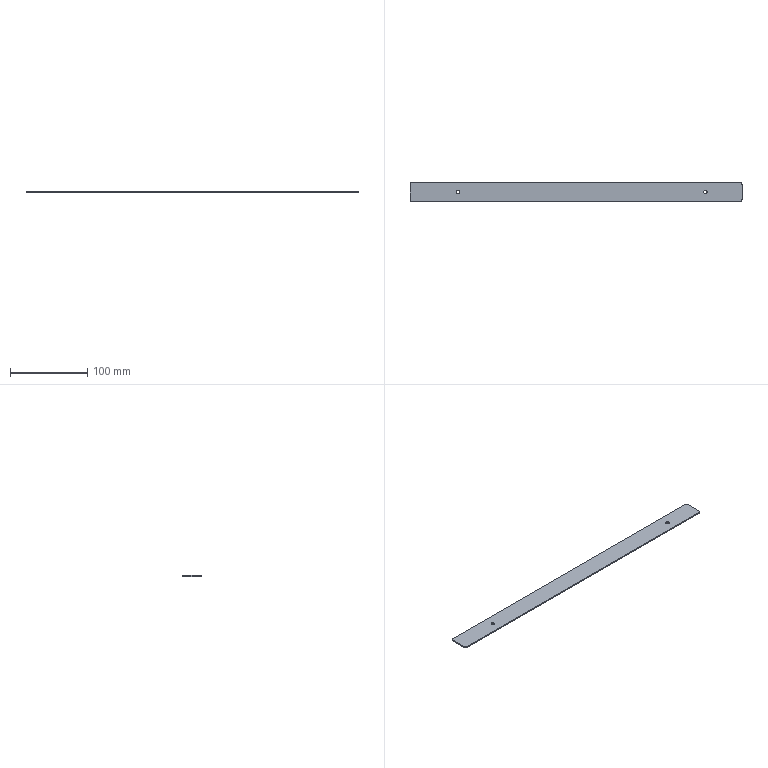Part | STEP file | 1 solid | 14 faces | box 430 x 25 x 1.5 mm | volume 16066 mm3 | cylinder 8 | plane 6 | commonest cylinder face diameters 4.5 x4 6 x4
STEP:
#1=CARTESIAN_POINT('',(0.,0.,0.));
#2=DIRECTION('',(0.,0.,1.));
#3=DIRECTION('',(1.,0.,0.));
#4=AXIS2_PLACEMENT_3D('',#1,#2,#3);
#5=CARTESIAN_POINT('',(-108.085,-48.,1.5));
#6=VERTEX_POINT('',#5);
#7=CARTESIAN_POINT('',(-111.085,-45.,1.5));
#8=VERTEX_POINT('',#7);
#9=CARTESIAN_POINT('',(-111.085,-48.,1.5));
#10=DIRECTION('',(0.,0.,1.));
#11=DIRECTION('',(1.,0.,0.));
#12=AXIS2_PLACEMENT_3D('',#9,#10,#11);
#13=CIRCLE('',#12,3.);
#14=CARTESIAN_POINT('',(-111.085,-48.,1.5));
#15=DIRECTION('',(0.,0.,-1.));
#16=DIRECTION('',(-1.,0.,0.));
#17=AXIS2_PLACEMENT_3D('',#14,#15,#16);
#18=CYLINDRICAL_SURFACE('',#17,3.);
#19=CARTESIAN_POINT('',(3.142,0.));
#20=DIRECTION('',(-1.,0.));
#21=VECTOR('',#20,1.);
#22=LINE('',#19,#21);
#23=(GEOMETRIC_REPRESENTATION_CONTEXT(2)PARAMETRIC_REPRESENTATION_CONTEXT()REPRESENTATION_CONTEXT('',''));
#24=DEFINITIONAL_REPRESENTATION('',(#22),#23);
#25=PCURVE('',#18,#24);
#26=CARTESIAN_POINT('',(0.,0.,1.5));
#27=DIRECTION('',(0.,0.,1.));
#28=DIRECTION('',(1.,0.,0.));
#29=AXIS2_PLACEMENT_3D('',#26,#27,#28);
#30=PLANE('',#29);
#31=CARTESIAN_POINT('',(-111.085,-48.));
#32=DIRECTION('',(1.,0.));
#33=AXIS2_PLACEMENT_2D('',#31,#32);
#34=CIRCLE('',#33,3.);
#35=(GEOMETRIC_REPRESENTATION_CONTEXT(2)PARAMETRIC_REPRESENTATION_CONTEXT()REPRESENTATION_CONTEXT('',''));
#36=DEFINITIONAL_REPRESENTATION('',(#34),#35);
#37=PCURVE('',#30,#36);
#38=SURFACE_CURVE('',#13,(#25,#37),.PCURVE_S1.);
#39=EDGE_CURVE('',#6,#8,#38,.T.);
#40=ORIENTED_EDGE('',*,*,#39,.F.);
#41=CARTESIAN_POINT('',(-108.085,-48.,0.));
#42=VERTEX_POINT('',#41);
#43=CARTESIAN_POINT('',(-108.085,-48.,1.5));
#44=DIRECTION('',(0.,0.,1.));
#45=VECTOR('',#44,1.);
#46=LINE('',#43,#45);
#47=CARTESIAN_POINT('',(3.142,0.));
#48=DIRECTION('',(0.,-1.));
#49=VECTOR('',#48,1.);
#50=LINE('',#47,#49);
#51=(GEOMETRIC_REPRESENTATION_CONTEXT(2)PARAMETRIC_REPRESENTATION_CONTEXT()REPRESENTATION_CONTEXT('',''));
#52=DEFINITIONAL_REPRESENTATION('',(#50),#51);
#53=PCURVE('',#18,#52);
#54=CARTESIAN_POINT('',(-108.085,-70.,1.5));
#55=DIRECTION('',(-1.,0.,0.));
#56=DIRECTION('',(0.,0.,1.));
#57=AXIS2_PLACEMENT_3D('',#54,#55,#56);
#58=PLANE('',#57);
#59=CARTESIAN_POINT('',(0.,22.));
#60=DIRECTION('',(1.,0.));
#61=VECTOR('',#60,1.);
#62=LINE('',#59,#61);
#63=(GEOMETRIC_REPRESENTATION_CONTEXT(2)PARAMETRIC_REPRESENTATION_CONTEXT()REPRESENTATION_CONTEXT('',''));
#64=DEFINITIONAL_REPRESENTATION('',(#62),#63);
#65=PCURVE('',#58,#64);
#66=SURFACE_CURVE('',#46,(#53,#65),.PCURVE_S1.);
#67=EDGE_CURVE('',#42,#6,#66,.T.);
#68=ORIENTED_EDGE('',*,*,#67,.F.);
#69=CARTESIAN_POINT('',(-111.085,-45.,0.));
#70=VERTEX_POINT('',#69);
#71=CARTESIAN_POINT('',(-111.085,-48.,0.));
#72=DIRECTION('',(0.,0.,-1.));
#73=DIRECTION('',(1.,0.,0.));
#74=AXIS2_PLACEMENT_3D('',#71,#72,#73);
#75=CIRCLE('',#74,3.);
#76=CARTESIAN_POINT('',(-3.142,1.5));
#77=DIRECTION('',(1.,0.));
#78=VECTOR('',#77,1.);
#79=LINE('',#76,#78);
#80=(GEOMETRIC_REPRESENTATION_CONTEXT(2)PARAMETRIC_REPRESENTATION_CONTEXT()REPRESENTATION_CONTEXT('',''));
#81=DEFINITIONAL_REPRESENTATION('',(#79),#80);
#82=PCURVE('',#18,#81);
#83=CARTESIAN_POINT('',(0.,0.,0.));
#84=DIRECTION('',(0.,0.,1.));
#85=DIRECTION('',(1.,0.,0.));
#86=AXIS2_PLACEMENT_3D('',#83,#84,#85);
#87=PLANE('',#86);
#88=CARTESIAN_POINT('',(-108.085,-48.));
#89=CARTESIAN_POINT('',(-108.085,-53.196));
#90=CARTESIAN_POINT('',(-112.585,-50.598));
#91=CARTESIAN_POINT('',(-117.085,-48.));
#92=CARTESIAN_POINT('',(-112.585,-45.402));
#93=CARTESIAN_POINT('',(-108.085,-42.804));
#94=CARTESIAN_POINT('',(-108.085,-48.));
#95=(BOUNDED_CURVE()B_SPLINE_CURVE(2,(#88,#89,#90,#91,#92,#93,#94),.UNSPECIFIED.,.T.,.F.)B_SPLINE_CURVE_WITH_KNOTS((1,2,2,2,2,1),(-2.094,0.,2.094,4.189,6.283,8.378),.UNSPECIFIED.)CURVE()GEOMETRIC_REPRESENTATION_ITEM()RATIONAL_B_SPLINE_CURVE((1.,0.5,1.,0.5,1.,0.5,1.))REPRESENTATION_ITEM(''));
#96=(GEOMETRIC_REPRESENTATION_CONTEXT(2)PARAMETRIC_REPRESENTATION_CONTEXT()REPRESENTATION_CONTEXT('',''));
#97=DEFINITIONAL_REPRESENTATION('',(#95),#96);
#98=PCURVE('',#87,#97);
#99=SURFACE_CURVE('',#75,(#82,#98),.PCURVE_S1.);
#100=EDGE_CURVE('',#70,#42,#99,.T.);
#101=ORIENTED_EDGE('',*,*,#100,.F.);
#102=CARTESIAN_POINT('',(-111.085,-45.,1.5));
#103=DIRECTION('',(0.,0.,-1.));
#104=VECTOR('',#103,1.);
#105=LINE('',#102,#104);
#106=CARTESIAN_POINT('',(1.571,0.));
#107=DIRECTION('',(0.,1.));
#108=VECTOR('',#107,1.);
#109=LINE('',#106,#108);
#110=(GEOMETRIC_REPRESENTATION_CONTEXT(2)PARAMETRIC_REPRESENTATION_CONTEXT()REPRESENTATION_CONTEXT('',''));
#111=DEFINITIONAL_REPRESENTATION('',(#109),#110);
#112=PCURVE('',#18,#111);
#113=CARTESIAN_POINT('',(-108.085,-45.,1.5));
#114=DIRECTION('',(0.,-1.,0.));
#115=DIRECTION('',(-1.,0.,0.));
#116=AXIS2_PLACEMENT_3D('',#113,#114,#115);
#117=PLANE('',#116);
#118=CARTESIAN_POINT('',(3.,0.));
#119=DIRECTION('',(0.,1.));
#120=VECTOR('',#119,1.);
#121=LINE('',#118,#120);
#122=(GEOMETRIC_REPRESENTATION_CONTEXT(2)PARAMETRIC_REPRESENTATION_CONTEXT()REPRESENTATION_CONTEXT('',''));
#123=DEFINITIONAL_REPRESENTATION('',(#121),#122);
#124=PCURVE('',#117,#123);
#125=SURFACE_CURVE('',#105,(#112,#124),.PCURVE_S1.);
#126=EDGE_CURVE('',#8,#70,#125,.T.);
#127=ORIENTED_EDGE('',*,*,#126,.F.);
#128=EDGE_LOOP('',(#40,#68,#101,#127));
#129=FACE_BOUND('',#128,.T.);
#130=ADVANCED_FACE('',(#129),#18,.T.);
#131=CARTESIAN_POINT('',(-111.085,-70.,1.5));
#132=VERTEX_POINT('',#131);
#133=CARTESIAN_POINT('',(-108.085,-67.,1.5));
#134=VERTEX_POINT('',#133);
#135=CARTESIAN_POINT('',(-111.085,-67.,1.5));
#136=DIRECTION('',(0.,0.,1.));
#137=DIRECTION('',(1.,0.,0.));
#138=AXIS2_PLACEMENT_3D('',#135,#136,#137);
#139=CIRCLE('',#138,3.);
#140=CARTESIAN_POINT('',(-111.085,-67.,1.5));
#141=DIRECTION('',(0.,0.,-1.));
#142=DIRECTION('',(-1.,0.,0.));
#143=AXIS2_PLACEMENT_3D('',#140,#141,#142);
#144=CYLINDRICAL_SURFACE('',#143,3.);
#145=CARTESIAN_POINT('',(9.425,0.));
#146=DIRECTION('',(-1.,0.));
#147=VECTOR('',#146,1.);
#148=LINE('',#145,#147);
#149=(GEOMETRIC_REPRESENTATION_CONTEXT(2)PARAMETRIC_REPRESENTATION_CONTEXT()REPRESENTATION_CONTEXT('',''));
#150=DEFINITIONAL_REPRESENTATION('',(#148),#149);
#151=PCURVE('',#144,#150);
#152=CARTESIAN_POINT('',(-111.085,-67.));
#153=DIRECTION('',(1.,0.));
#154=AXIS2_PLACEMENT_2D('',#152,#153);
#155=CIRCLE('',#154,3.);
#156=(GEOMETRIC_REPRESENTATION_CONTEXT(2)PARAMETRIC_REPRESENTATION_CONTEXT()REPRESENTATION_CONTEXT('',''));
#157=DEFINITIONAL_REPRESENTATION('',(#155),#156);
#158=PCURVE('',#30,#157);
#159=SURFACE_CURVE('',#139,(#151,#158),.PCURVE_S1.);
#160=EDGE_CURVE('',#132,#134,#159,.T.);
#161=ORIENTED_EDGE('',*,*,#160,.F.);
#162=CARTESIAN_POINT('',(-111.085,-70.,0.));
#163=VERTEX_POINT('',#162);
#164=CARTESIAN_POINT('',(-111.085,-70.,1.5));
#165=DIRECTION('',(0.,0.,1.));
#166=VECTOR('',#165,1.);
#167=LINE('',#164,#166);
#168=CARTESIAN_POINT('',(4.712,0.));
#169=DIRECTION('',(0.,-1.));
#170=VECTOR('',#169,1.);
#171=LINE('',#168,#170);
#172=(GEOMETRIC_REPRESENTATION_CONTEXT(2)PARAMETRIC_REPRESENTATION_CONTEXT()REPRESENTATION_CONTEXT('',''));
#173=DEFINITIONAL_REPRESENTATION('',(#171),#172);
#174=PCURVE('',#144,#173);
#175=CARTESIAN_POINT('',(-558.085,-70.,1.5));
#176=DIRECTION('',(0.,1.,0.));
#177=DIRECTION('',(1.,0.,0.));
#178=AXIS2_PLACEMENT_3D('',#175,#176,#177);
#179=PLANE('',#178);
#180=CARTESIAN_POINT('',(447.,0.));
#181=DIRECTION('',(0.,-1.));
#182=VECTOR('',#181,1.);
#183=LINE('',#180,#182);
#184=(GEOMETRIC_REPRESENTATION_CONTEXT(2)PARAMETRIC_REPRESENTATION_CONTEXT()REPRESENTATION_CONTEXT('',''));
#185=DEFINITIONAL_REPRESENTATION('',(#183),#184);
#186=PCURVE('',#179,#185);
#187=SURFACE_CURVE('',#167,(#174,#186),.PCURVE_S1.);
#188=EDGE_CURVE('',#163,#132,#187,.T.);
#189=ORIENTED_EDGE('',*,*,#188,.F.);
#190=CARTESIAN_POINT('',(-108.085,-67.,0.));
#191=VERTEX_POINT('',#190);
#192=CARTESIAN_POINT('',(-111.085,-67.,0.));
#193=DIRECTION('',(0.,0.,-1.));
#194=DIRECTION('',(1.,0.,0.));
#195=AXIS2_PLACEMENT_3D('',#192,#193,#194);
#196=CIRCLE('',#195,3.);
#197=CARTESIAN_POINT('',(3.142,1.5));
#198=DIRECTION('',(1.,0.));
#199=VECTOR('',#198,1.);
#200=LINE('',#197,#199);
#201=(GEOMETRIC_REPRESENTATION_CONTEXT(2)PARAMETRIC_REPRESENTATION_CONTEXT()REPRESENTATION_CONTEXT('',''));
#202=DEFINITIONAL_REPRESENTATION('',(#200),#201);
#203=PCURVE('',#144,#202);
#204=CARTESIAN_POINT('',(-108.085,-67.));
#205=CARTESIAN_POINT('',(-108.085,-72.196));
#206=CARTESIAN_POINT('',(-112.585,-69.598));
#207=CARTESIAN_POINT('',(-117.085,-67.));
#208=CARTESIAN_POINT('',(-112.585,-64.402));
#209=CARTESIAN_POINT('',(-108.085,-61.804));
#210=CARTESIAN_POINT('',(-108.085,-67.));
#211=(BOUNDED_CURVE()B_SPLINE_CURVE(2,(#204,#205,#206,#207,#208,#209,#210),.UNSPECIFIED.,.T.,.F.)B_SPLINE_CURVE_WITH_KNOTS((1,2,2,2,2,1),(-2.094,0.,2.094,4.189,6.283,8.378),.UNSPECIFIED.)CURVE()GEOMETRIC_REPRESENTATION_ITEM()RATIONAL_B_SPLINE_CURVE((1.,0.5,1.,0.5,1.,0.5,1.))REPRESENTATION_ITEM(''));
#212=(GEOMETRIC_REPRESENTATION_CONTEXT(2)PARAMETRIC_REPRESENTATION_CONTEXT()REPRESENTATION_CONTEXT('',''));
#213=DEFINITIONAL_REPRESENTATION('',(#211),#212);
#214=PCURVE('',#87,#213);
#215=SURFACE_CURVE('',#196,(#203,#214),.PCURVE_S1.);
#216=EDGE_CURVE('',#191,#163,#215,.T.);
#217=ORIENTED_EDGE('',*,*,#216,.F.);
#218=CARTESIAN_POINT('',(-108.085,-67.,1.5));
#219=DIRECTION('',(0.,0.,-1.));
#220=VECTOR('',#219,1.);
#221=LINE('',#218,#220);
#222=CARTESIAN_POINT('',(3.142,0.));
#223=DIRECTION('',(0.,1.));
#224=VECTOR('',#223,1.);
#225=LINE('',#222,#224);
#226=(GEOMETRIC_REPRESENTATION_CONTEXT(2)PARAMETRIC_REPRESENTATION_CONTEXT()REPRESENTATION_CONTEXT('',''));
#227=DEFINITIONAL_REPRESENTATION('',(#225),#226);
#228=PCURVE('',#144,#227);
#229=CARTESIAN_POINT('',(0.,3.));
#230=DIRECTION('',(-1.,0.));
#231=VECTOR('',#230,1.);
#232=LINE('',#229,#231);
#233=(GEOMETRIC_REPRESENTATION_CONTEXT(2)PARAMETRIC_REPRESENTATION_CONTEXT()REPRESENTATION_CONTEXT('',''));
#234=DEFINITIONAL_REPRESENTATION('',(#232),#233);
#235=PCURVE('',#58,#234);
#236=SURFACE_CURVE('',#221,(#228,#235),.PCURVE_S1.);
#237=EDGE_CURVE('',#134,#191,#236,.T.);
#238=ORIENTED_EDGE('',*,*,#237,.F.);
#239=EDGE_LOOP('',(#161,#189,#217,#238));
#240=FACE_BOUND('',#239,.T.);
#241=ADVANCED_FACE('',(#240),#144,.T.);
#242=CARTESIAN_POINT('',(-535.085,-45.,1.5));
#243=VERTEX_POINT('',#242);
#244=CARTESIAN_POINT('',(-538.085,-48.,1.5));
#245=VERTEX_POINT('',#244);
#246=CARTESIAN_POINT('',(-535.085,-48.,1.5));
#247=DIRECTION('',(0.,0.,1.));
#248=DIRECTION('',(1.,0.,0.));
#249=AXIS2_PLACEMENT_3D('',#246,#247,#248);
#250=CIRCLE('',#249,3.);
#251=CARTESIAN_POINT('',(-535.085,-48.,1.5));
#252=DIRECTION('',(0.,0.,-1.));
#253=DIRECTION('',(-1.,0.,0.));
#254=AXIS2_PLACEMENT_3D('',#251,#252,#253);
#255=CYLINDRICAL_SURFACE('',#254,3.);
#256=CARTESIAN_POINT('',(3.142,0.));
#257=DIRECTION('',(-1.,0.));
#258=VECTOR('',#257,1.);
#259=LINE('',#256,#258);
#260=(GEOMETRIC_REPRESENTATION_CONTEXT(2)PARAMETRIC_REPRESENTATION_CONTEXT()REPRESENTATION_CONTEXT('',''));
#261=DEFINITIONAL_REPRESENTATION('',(#259),#260);
#262=PCURVE('',#255,#261);
#263=CARTESIAN_POINT('',(-535.085,-48.));
#264=DIRECTION('',(1.,0.));
#265=AXIS2_PLACEMENT_2D('',#263,#264);
#266=CIRCLE('',#265,3.);
#267=(GEOMETRIC_REPRESENTATION_CONTEXT(2)PARAMETRIC_REPRESENTATION_CONTEXT()REPRESENTATION_CONTEXT('',''));
#268=DEFINITIONAL_REPRESENTATION('',(#266),#267);
#269=PCURVE('',#30,#268);
#270=SURFACE_CURVE('',#250,(#262,#269),.PCURVE_S1.);
#271=EDGE_CURVE('',#243,#245,#270,.T.);
#272=ORIENTED_EDGE('',*,*,#271,.F.);
#273=CARTESIAN_POINT('',(-535.085,-45.,0.));
#274=VERTEX_POINT('',#273);
#275=CARTESIAN_POINT('',(-535.085,-45.,1.5));
#276=DIRECTION('',(0.,0.,1.));
#277=VECTOR('',#276,1.);
#278=LINE('',#275,#277);
#279=CARTESIAN_POINT('',(1.571,0.));
#280=DIRECTION('',(0.,-1.));
#281=VECTOR('',#280,1.);
#282=LINE('',#279,#281);
#283=(GEOMETRIC_REPRESENTATION_CONTEXT(2)PARAMETRIC_REPRESENTATION_CONTEXT()REPRESENTATION_CONTEXT('',''));
#284=DEFINITIONAL_REPRESENTATION('',(#282),#283);
#285=PCURVE('',#255,#284);
#286=CARTESIAN_POINT('',(427.,0.));
#287=DIRECTION('',(0.,-1.));
#288=VECTOR('',#287,1.);
#289=LINE('',#286,#288);
#290=(GEOMETRIC_REPRESENTATION_CONTEXT(2)PARAMETRIC_REPRESENTATION_CONTEXT()REPRESENTATION_CONTEXT('',''));
#291=DEFINITIONAL_REPRESENTATION('',(#289),#290);
#292=PCURVE('',#117,#291);
#293=SURFACE_CURVE('',#278,(#285,#292),.PCURVE_S1.);
#294=EDGE_CURVE('',#274,#243,#293,.T.);
#295=ORIENTED_EDGE('',*,*,#294,.F.);
#296=CARTESIAN_POINT('',(-538.085,-48.,0.));
#297=VERTEX_POINT('',#296);
#298=CARTESIAN_POINT('',(-535.085,-48.,0.));
#299=DIRECTION('',(0.,0.,-1.));
#300=DIRECTION('',(1.,0.,0.));
#301=AXIS2_PLACEMENT_3D('',#298,#299,#300);
#302=CIRCLE('',#301,3.);
#303=CARTESIAN_POINT('',(-3.142,1.5));
#304=DIRECTION('',(1.,0.));
#305=VECTOR('',#304,1.);
#306=LINE('',#303,#305);
#307=(GEOMETRIC_REPRESENTATION_CONTEXT(2)PARAMETRIC_REPRESENTATION_CONTEXT()REPRESENTATION_CONTEXT('',''));
#308=DEFINITIONAL_REPRESENTATION('',(#306),#307);
#309=PCURVE('',#255,#308);
#310=CARTESIAN_POINT('',(-532.085,-48.));
#311=CARTESIAN_POINT('',(-532.085,-53.196));
#312=CARTESIAN_POINT('',(-536.585,-50.598));
#313=CARTESIAN_POINT('',(-541.085,-48.));
#314=CARTESIAN_POINT('',(-536.585,-45.402));
#315=CARTESIAN_POINT('',(-532.085,-42.804));
#316=CARTESIAN_POINT('',(-532.085,-48.));
#317=(BOUNDED_CURVE()B_SPLINE_CURVE(2,(#310,#311,#312,#313,#314,#315,#316),.UNSPECIFIED.,.T.,.F.)B_SPLINE_CURVE_WITH_KNOTS((1,2,2,2,2,1),(-2.094,0.,2.094,4.189,6.283,8.378),.UNSPECIFIED.)CURVE()GEOMETRIC_REPRESENTATION_ITEM()RATIONAL_B_SPLINE_CURVE((1.,0.5,1.,0.5,1.,0.5,1.))REPRESENTATION_ITEM(''));
#318=(GEOMETRIC_REPRESENTATION_CONTEXT(2)PARAMETRIC_REPRESENTATION_CONTEXT()REPRESENTATION_CONTEXT('',''));
#319=DEFINITIONAL_REPRESENTATION('',(#317),#318);
#320=PCURVE('',#87,#319);
#321=SURFACE_CURVE('',#302,(#309,#320),.PCURVE_S1.);
#322=EDGE_CURVE('',#297,#274,#321,.T.);
#323=ORIENTED_EDGE('',*,*,#322,.F.);
#324=CARTESIAN_POINT('',(-538.085,-48.,1.5));
#325=DIRECTION('',(0.,0.,-1.));
#326=VECTOR('',#325,1.);
#327=LINE('',#324,#326);
#328=CARTESIAN_POINT('',(0.,0.));
#329=DIRECTION('',(0.,1.));
#330=VECTOR('',#329,1.);
#331=LINE('',#328,#330);
#332=(GEOMETRIC_REPRESENTATION_CONTEXT(2)PARAMETRIC_REPRESENTATION_CONTEXT()REPRESENTATION_CONTEXT('',''));
#333=DEFINITIONAL_REPRESENTATION('',(#331),#332);
#334=PCURVE('',#255,#333);
#335=CARTESIAN_POINT('',(-538.085,-45.,1.5));
#336=DIRECTION('',(1.,0.,0.));
#337=DIRECTION('',(0.,1.,0.));
#338=AXIS2_PLACEMENT_3D('',#335,#336,#337);
#339=PLANE('',#338);
#340=CARTESIAN_POINT('',(-3.,0.));
#341=DIRECTION('',(0.,-1.));
#342=VECTOR('',#341,1.);
#343=LINE('',#340,#342);
#344=(GEOMETRIC_REPRESENTATION_CONTEXT(2)PARAMETRIC_REPRESENTATION_CONTEXT()REPRESENTATION_CONTEXT('',''));
#345=DEFINITIONAL_REPRESENTATION('',(#343),#344);
#346=PCURVE('',#339,#345);
#347=SURFACE_CURVE('',#327,(#334,#346),.PCURVE_S1.);
#348=EDGE_CURVE('',#245,#297,#347,.T.);
#349=ORIENTED_EDGE('',*,*,#348,.F.);
#350=EDGE_LOOP('',(#272,#295,#323,#349));
#351=FACE_BOUND('',#350,.T.);
#352=ADVANCED_FACE('',(#351),#255,.T.);
#353=CARTESIAN_POINT('',(-538.085,-67.,1.5));
#354=VERTEX_POINT('',#353);
#355=CARTESIAN_POINT('',(-535.085,-70.,1.5));
#356=VERTEX_POINT('',#355);
#357=CARTESIAN_POINT('',(-535.085,-67.,1.5));
#358=DIRECTION('',(0.,0.,1.));
#359=DIRECTION('',(1.,0.,0.));
#360=AXIS2_PLACEMENT_3D('',#357,#358,#359);
#361=CIRCLE('',#360,3.);
#362=CARTESIAN_POINT('',(-535.085,-67.,1.5));
#363=DIRECTION('',(0.,0.,-1.));
#364=DIRECTION('',(-1.,0.,0.));
#365=AXIS2_PLACEMENT_3D('',#362,#363,#364);
#366=CYLINDRICAL_SURFACE('',#365,3.);
#367=CARTESIAN_POINT('',(9.425,0.));
#368=DIRECTION('',(-1.,0.));
#369=VECTOR('',#368,1.);
#370=LINE('',#367,#369);
#371=(GEOMETRIC_REPRESENTATION_CONTEXT(2)PARAMETRIC_REPRESENTATION_CONTEXT()REPRESENTATION_CONTEXT('',''));
#372=DEFINITIONAL_REPRESENTATION('',(#370),#371);
#373=PCURVE('',#366,#372);
#374=CARTESIAN_POINT('',(-535.085,-67.));
#375=DIRECTION('',(1.,0.));
#376=AXIS2_PLACEMENT_2D('',#374,#375);
#377=CIRCLE('',#376,3.);
#378=(GEOMETRIC_REPRESENTATION_CONTEXT(2)PARAMETRIC_REPRESENTATION_CONTEXT()REPRESENTATION_CONTEXT('',''));
#379=DEFINITIONAL_REPRESENTATION('',(#377),#378);
#380=PCURVE('',#30,#379);
#381=SURFACE_CURVE('',#361,(#373,#380),.PCURVE_S1.);
#382=EDGE_CURVE('',#354,#356,#381,.T.);
#383=ORIENTED_EDGE('',*,*,#382,.F.);
#384=CARTESIAN_POINT('',(-538.085,-67.,0.));
#385=VERTEX_POINT('',#384);
#386=CARTESIAN_POINT('',(-538.085,-67.,1.5));
#387=DIRECTION('',(0.,0.,1.));
#388=VECTOR('',#387,1.);
#389=LINE('',#386,#388);
#390=CARTESIAN_POINT('',(6.283,0.));
#391=DIRECTION('',(0.,-1.));
#392=VECTOR('',#391,1.);
#393=LINE('',#390,#392);
#394=(GEOMETRIC_REPRESENTATION_CONTEXT(2)PARAMETRIC_REPRESENTATION_CONTEXT()REPRESENTATION_CONTEXT('',''));
#395=DEFINITIONAL_REPRESENTATION('',(#393),#394);
#396=PCURVE('',#366,#395);
#397=CARTESIAN_POINT('',(-22.,0.));
#398=DIRECTION('',(0.,1.));
#399=VECTOR('',#398,1.);
#400=LINE('',#397,#399);
#401=(GEOMETRIC_REPRESENTATION_CONTEXT(2)PARAMETRIC_REPRESENTATION_CONTEXT()REPRESENTATION_CONTEXT('',''));
#402=DEFINITIONAL_REPRESENTATION('',(#400),#401);
#403=PCURVE('',#339,#402);
#404=SURFACE_CURVE('',#389,(#396,#403),.PCURVE_S1.);
#405=EDGE_CURVE('',#385,#354,#404,.T.);
#406=ORIENTED_EDGE('',*,*,#405,.F.);
#407=CARTESIAN_POINT('',(-535.085,-70.,0.));
#408=VERTEX_POINT('',#407);
#409=CARTESIAN_POINT('',(-535.085,-67.,0.));
#410=DIRECTION('',(0.,0.,-1.));
#411=DIRECTION('',(1.,0.,0.));
#412=AXIS2_PLACEMENT_3D('',#409,#410,#411);
#413=CIRCLE('',#412,3.);
#414=CARTESIAN_POINT('',(3.142,1.5));
#415=DIRECTION('',(1.,0.));
#416=VECTOR('',#415,1.);
#417=LINE('',#414,#416);
#418=(GEOMETRIC_REPRESENTATION_CONTEXT(2)PARAMETRIC_REPRESENTATION_CONTEXT()REPRESENTATION_CONTEXT('',''));
#419=DEFINITIONAL_REPRESENTATION('',(#417),#418);
#420=PCURVE('',#366,#419);
#421=CARTESIAN_POINT('',(-532.085,-67.));
#422=CARTESIAN_POINT('',(-532.085,-72.196));
#423=CARTESIAN_POINT('',(-536.585,-69.598));
#424=CARTESIAN_POINT('',(-541.085,-67.));
#425=CARTESIAN_POINT('',(-536.585,-64.402));
#426=CARTESIAN_POINT('',(-532.085,-61.804));
#427=CARTESIAN_POINT('',(-532.085,-67.));
#428=(BOUNDED_CURVE()B_SPLINE_CURVE(2,(#421,#422,#423,#424,#425,#426,#427),.UNSPECIFIED.,.T.,.F.)B_SPLINE_CURVE_WITH_KNOTS((1,2,2,2,2,1),(-2.094,0.,2.094,4.189,6.283,8.378),.UNSPECIFIED.)CURVE()GEOMETRIC_REPRESENTATION_ITEM()RATIONAL_B_SPLINE_CURVE((1.,0.5,1.,0.5,1.,0.5,1.))REPRESENTATION_ITEM(''));
#429=(GEOMETRIC_REPRESENTATION_CONTEXT(2)PARAMETRIC_REPRESENTATION_CONTEXT()REPRESENTATION_CONTEXT('',''));
#430=DEFINITIONAL_REPRESENTATION('',(#428),#429);
#431=PCURVE('',#87,#430);
#432=SURFACE_CURVE('',#413,(#420,#431),.PCURVE_S1.);
#433=EDGE_CURVE('',#408,#385,#432,.T.);
#434=ORIENTED_EDGE('',*,*,#433,.F.);
#435=CARTESIAN_POINT('',(-535.085,-70.,1.5));
#436=DIRECTION('',(0.,0.,-1.));
#437=VECTOR('',#436,1.);
#438=LINE('',#435,#437);
#439=CARTESIAN_POINT('',(4.712,0.));
#440=DIRECTION('',(0.,1.));
#441=VECTOR('',#440,1.);
#442=LINE('',#439,#441);
#443=(GEOMETRIC_REPRESENTATION_CONTEXT(2)PARAMETRIC_REPRESENTATION_CONTEXT()REPRESENTATION_CONTEXT('',''));
#444=DEFINITIONAL_REPRESENTATION('',(#442),#443);
#445=PCURVE('',#366,#444);
#446=CARTESIAN_POINT('',(23.,0.));
#447=DIRECTION('',(0.,1.));
#448=VECTOR('',#447,1.);
#449=LINE('',#446,#448);
#450=(GEOMETRIC_REPRESENTATION_CONTEXT(2)PARAMETRIC_REPRESENTATION_CONTEXT()REPRESENTATION_CONTEXT('',''));
#451=DEFINITIONAL_REPRESENTATION('',(#449),#450);
#452=PCURVE('',#179,#451);
#453=SURFACE_CURVE('',#438,(#445,#452),.PCURVE_S1.);
#454=EDGE_CURVE('',#356,#408,#453,.T.);
#455=ORIENTED_EDGE('',*,*,#454,.F.);
#456=EDGE_LOOP('',(#383,#406,#434,#455));
#457=FACE_BOUND('',#456,.T.);
#458=ADVANCED_FACE('',(#457),#366,.T.);
#459=CARTESIAN_POINT('',(-153.335,-57.5,1.5));
#460=VERTEX_POINT('',#459);
#461=CARTESIAN_POINT('',(-157.835,-57.5,1.5));
#462=VERTEX_POINT('',#461);
#463=CARTESIAN_POINT('',(-155.585,-57.5,1.5));
#464=DIRECTION('',(0.,0.,1.));
#465=DIRECTION('',(1.,0.,0.));
#466=AXIS2_PLACEMENT_3D('',#463,#464,#465);
#467=CIRCLE('',#466,2.25);
#468=CARTESIAN_POINT('',(-155.585,-57.5,1.5));
#469=DIRECTION('',(0.,0.,1.));
#470=DIRECTION('',(1.,0.,0.));
#471=AXIS2_PLACEMENT_3D('',#468,#469,#470);
#472=CYLINDRICAL_SURFACE('',#471,2.25);
#473=CARTESIAN_POINT('',(0.,0.));
#474=DIRECTION('',(1.,0.));
#475=VECTOR('',#474,1.);
#476=LINE('',#473,#475);
#477=(GEOMETRIC_REPRESENTATION_CONTEXT(2)PARAMETRIC_REPRESENTATION_CONTEXT()REPRESENTATION_CONTEXT('',''));
#478=DEFINITIONAL_REPRESENTATION('',(#476),#477);
#479=PCURVE('',#472,#478);
#480=CARTESIAN_POINT('',(-155.585,-57.5));
#481=DIRECTION('',(1.,0.));
#482=AXIS2_PLACEMENT_2D('',#480,#481);
#483=CIRCLE('',#482,2.25);
#484=(GEOMETRIC_REPRESENTATION_CONTEXT(2)PARAMETRIC_REPRESENTATION_CONTEXT()REPRESENTATION_CONTEXT('',''));
#485=DEFINITIONAL_REPRESENTATION('',(#483),#484);
#486=PCURVE('',#30,#485);
#487=SURFACE_CURVE('',#467,(#479,#486),.PCURVE_S1.);
#488=EDGE_CURVE('',#460,#462,#487,.T.);
#489=ORIENTED_EDGE('',*,*,#488,.F.);
#490=CARTESIAN_POINT('',(-153.335,-57.5,0.));
#491=VERTEX_POINT('',#490);
#492=CARTESIAN_POINT('',(-153.335,-57.5,1.5));
#493=DIRECTION('',(0.,0.,1.));
#494=VECTOR('',#493,1.);
#495=LINE('',#492,#494);
#496=CARTESIAN_POINT('',(0.,0.));
#497=DIRECTION('',(0.,1.));
#498=VECTOR('',#497,1.);
#499=LINE('',#496,#498);
#500=(GEOMETRIC_REPRESENTATION_CONTEXT(2)PARAMETRIC_REPRESENTATION_CONTEXT()REPRESENTATION_CONTEXT('',''));
#501=DEFINITIONAL_REPRESENTATION('',(#499),#500);
#502=PCURVE('',#472,#501);
#503=CARTESIAN_POINT('',(-155.585,-57.5,1.5));
#504=DIRECTION('',(0.,0.,1.));
#505=DIRECTION('',(1.,0.,0.));
#506=AXIS2_PLACEMENT_3D('',#503,#504,#505);
#507=CYLINDRICAL_SURFACE('',#506,2.25);
#508=CARTESIAN_POINT('',(6.283,0.));
#509=DIRECTION('',(0.,1.));
#510=VECTOR('',#509,1.);
#511=LINE('',#508,#510);
#512=(GEOMETRIC_REPRESENTATION_CONTEXT(2)PARAMETRIC_REPRESENTATION_CONTEXT()REPRESENTATION_CONTEXT('',''));
#513=DEFINITIONAL_REPRESENTATION('',(#511),#512);
#514=PCURVE('',#507,#513);
#515=SURFACE_CURVE('',#495,(#502,#514),.PCURVE_S1.);
#516=EDGE_CURVE('',#491,#460,#515,.T.);
#517=ORIENTED_EDGE('',*,*,#516,.F.);
#518=CARTESIAN_POINT('',(-157.835,-57.5,0.));
#519=VERTEX_POINT('',#518);
#520=CARTESIAN_POINT('',(-155.585,-57.5,0.));
#521=DIRECTION('',(0.,0.,1.));
#522=DIRECTION('',(1.,0.,0.));
#523=AXIS2_PLACEMENT_3D('',#520,#521,#522);
#524=CIRCLE('',#523,2.25);
#525=CARTESIAN_POINT('',(0.,-1.5));
#526=DIRECTION('',(1.,0.));
#527=VECTOR('',#526,1.);
#528=LINE('',#525,#527);
#529=(GEOMETRIC_REPRESENTATION_CONTEXT(2)PARAMETRIC_REPRESENTATION_CONTEXT()REPRESENTATION_CONTEXT('',''));
#530=DEFINITIONAL_REPRESENTATION('',(#528),#529);
#531=PCURVE('',#472,#530);
#532=CARTESIAN_POINT('',(-155.585,-57.5));
#533=DIRECTION('',(1.,0.));
#534=AXIS2_PLACEMENT_2D('',#532,#533);
#535=CIRCLE('',#534,2.25);
#536=(GEOMETRIC_REPRESENTATION_CONTEXT(2)PARAMETRIC_REPRESENTATION_CONTEXT()REPRESENTATION_CONTEXT('',''));
#537=DEFINITIONAL_REPRESENTATION('',(#535),#536);
#538=PCURVE('',#87,#537);
#539=SURFACE_CURVE('',#524,(#531,#538),.PCURVE_S1.);
#540=EDGE_CURVE('',#491,#519,#539,.T.);
#541=ORIENTED_EDGE('',*,*,#540,.T.);
#542=CARTESIAN_POINT('',(-157.835,-57.5,1.5));
#543=DIRECTION('',(0.,0.,1.));
#544=VECTOR('',#543,1.);
#545=LINE('',#542,#544);
#546=CARTESIAN_POINT('',(3.142,0.));
#547=DIRECTION('',(0.,1.));
#548=VECTOR('',#547,1.);
#549=LINE('',#546,#548);
#550=(GEOMETRIC_REPRESENTATION_CONTEXT(2)PARAMETRIC_REPRESENTATION_CONTEXT()REPRESENTATION_CONTEXT('',''));
#551=DEFINITIONAL_REPRESENTATION('',(#549),#550);
#552=PCURVE('',#472,#551);
#553=CARTESIAN_POINT('',(3.142,0.));
#554=DIRECTION('',(0.,1.));
#555=VECTOR('',#554,1.);
#556=LINE('',#553,#555);
#557=(GEOMETRIC_REPRESENTATION_CONTEXT(2)PARAMETRIC_REPRESENTATION_CONTEXT()REPRESENTATION_CONTEXT('',''));
#558=DEFINITIONAL_REPRESENTATION('',(#556),#557);
#559=PCURVE('',#507,#558);
#560=SURFACE_CURVE('',#545,(#552,#559),.PCURVE_S1.);
#561=EDGE_CURVE('',#519,#462,#560,.T.);
#562=ORIENTED_EDGE('',*,*,#561,.T.);
#563=EDGE_LOOP('',(#489,#517,#541,#562));
#564=FACE_BOUND('',#563,.F.);
#565=ADVANCED_FACE('',(#564),#472,.F.);
#566=CARTESIAN_POINT('',(-473.335,-57.5,1.5));
#567=VERTEX_POINT('',#566);
#568=CARTESIAN_POINT('',(-477.835,-57.5,1.5));
#569=VERTEX_POINT('',#568);
#570=CARTESIAN_POINT('',(-475.585,-57.5,1.5));
#571=DIRECTION('',(0.,0.,1.));
#572=DIRECTION('',(1.,0.,0.));
#573=AXIS2_PLACEMENT_3D('',#570,#571,#572);
#574=CIRCLE('',#573,2.25);
#575=CARTESIAN_POINT('',(-475.585,-57.5,1.5));
#576=DIRECTION('',(0.,0.,1.));
#577=DIRECTION('',(1.,0.,0.));
#578=AXIS2_PLACEMENT_3D('',#575,#576,#577);
#579=CYLINDRICAL_SURFACE('',#578,2.25);
#580=CARTESIAN_POINT('',(0.,0.));
#581=DIRECTION('',(1.,0.));
#582=VECTOR('',#581,1.);
#583=LINE('',#580,#582);
#584=(GEOMETRIC_REPRESENTATION_CONTEXT(2)PARAMETRIC_REPRESENTATION_CONTEXT()REPRESENTATION_CONTEXT('',''));
#585=DEFINITIONAL_REPRESENTATION('',(#583),#584);
#586=PCURVE('',#579,#585);
#587=CARTESIAN_POINT('',(-475.585,-57.5));
#588=DIRECTION('',(1.,0.));
#589=AXIS2_PLACEMENT_2D('',#587,#588);
#590=CIRCLE('',#589,2.25);
#591=(GEOMETRIC_REPRESENTATION_CONTEXT(2)PARAMETRIC_REPRESENTATION_CONTEXT()REPRESENTATION_CONTEXT('',''));
#592=DEFINITIONAL_REPRESENTATION('',(#590),#591);
#593=PCURVE('',#30,#592);
#594=SURFACE_CURVE('',#574,(#586,#593),.PCURVE_S1.);
#595=EDGE_CURVE('',#567,#569,#594,.T.);
#596=ORIENTED_EDGE('',*,*,#595,.F.);
#597=CARTESIAN_POINT('',(-473.335,-57.5,0.));
#598=VERTEX_POINT('',#597);
#599=CARTESIAN_POINT('',(-473.335,-57.5,1.5));
#600=DIRECTION('',(0.,0.,1.));
#601=VECTOR('',#600,1.);
#602=LINE('',#599,#601);
#603=CARTESIAN_POINT('',(0.,0.));
#604=DIRECTION('',(0.,1.));
#605=VECTOR('',#604,1.);
#606=LINE('',#603,#605);
#607=(GEOMETRIC_REPRESENTATION_CONTEXT(2)PARAMETRIC_REPRESENTATION_CONTEXT()REPRESENTATION_CONTEXT('',''));
#608=DEFINITIONAL_REPRESENTATION('',(#606),#607);
#609=PCURVE('',#579,#608);
#610=CARTESIAN_POINT('',(-475.585,-57.5,1.5));
#611=DIRECTION('',(0.,0.,1.));
#612=DIRECTION('',(1.,0.,0.));
#613=AXIS2_PLACEMENT_3D('',#610,#611,#612);
#614=CYLINDRICAL_SURFACE('',#613,2.25);
#615=CARTESIAN_POINT('',(6.283,0.));
#616=DIRECTION('',(0.,1.));
#617=VECTOR('',#616,1.);
#618=LINE('',#615,#617);
#619=(GEOMETRIC_REPRESENTATION_CONTEXT(2)PARAMETRIC_REPRESENTATION_CONTEXT()REPRESENTATION_CONTEXT('',''));
#620=DEFINITIONAL_REPRESENTATION('',(#618),#619);
#621=PCURVE('',#614,#620);
#622=SURFACE_CURVE('',#602,(#609,#621),.PCURVE_S1.);
#623=EDGE_CURVE('',#598,#567,#622,.T.);
#624=ORIENTED_EDGE('',*,*,#623,.F.);
#625=CARTESIAN_POINT('',(-477.835,-57.5,0.));
#626=VERTEX_POINT('',#625);
#627=CARTESIAN_POINT('',(-475.585,-57.5,0.));
#628=DIRECTION('',(0.,0.,1.));
#629=DIRECTION('',(1.,0.,0.));
#630=AXIS2_PLACEMENT_3D('',#627,#628,#629);
#631=CIRCLE('',#630,2.25);
#632=CARTESIAN_POINT('',(0.,-1.5));
#633=DIRECTION('',(1.,0.));
#634=VECTOR('',#633,1.);
#635=LINE('',#632,#634);
#636=(GEOMETRIC_REPRESENTATION_CONTEXT(2)PARAMETRIC_REPRESENTATION_CONTEXT()REPRESENTATION_CONTEXT('',''));
#637=DEFINITIONAL_REPRESENTATION('',(#635),#636);
#638=PCURVE('',#579,#637);
#639=CARTESIAN_POINT('',(-475.585,-57.5));
#640=DIRECTION('',(1.,0.));
#641=AXIS2_PLACEMENT_2D('',#639,#640);
#642=CIRCLE('',#641,2.25);
#643=(GEOMETRIC_REPRESENTATION_CONTEXT(2)PARAMETRIC_REPRESENTATION_CONTEXT()REPRESENTATION_CONTEXT('',''));
#644=DEFINITIONAL_REPRESENTATION('',(#642),#643);
#645=PCURVE('',#87,#644);
#646=SURFACE_CURVE('',#631,(#638,#645),.PCURVE_S1.);
#647=EDGE_CURVE('',#598,#626,#646,.T.);
#648=ORIENTED_EDGE('',*,*,#647,.T.);
#649=CARTESIAN_POINT('',(-477.835,-57.5,1.5));
#650=DIRECTION('',(0.,0.,1.));
#651=VECTOR('',#650,1.);
#652=LINE('',#649,#651);
#653=CARTESIAN_POINT('',(3.142,0.));
#654=DIRECTION('',(0.,1.));
#655=VECTOR('',#654,1.);
#656=LINE('',#653,#655);
#657=(GEOMETRIC_REPRESENTATION_CONTEXT(2)PARAMETRIC_REPRESENTATION_CONTEXT()REPRESENTATION_CONTEXT('',''));
#658=DEFINITIONAL_REPRESENTATION('',(#656),#657);
#659=PCURVE('',#579,#658);
#660=CARTESIAN_POINT('',(3.142,0.));
#661=DIRECTION('',(0.,1.));
#662=VECTOR('',#661,1.);
#663=LINE('',#660,#662);
#664=(GEOMETRIC_REPRESENTATION_CONTEXT(2)PARAMETRIC_REPRESENTATION_CONTEXT()REPRESENTATION_CONTEXT('',''));
#665=DEFINITIONAL_REPRESENTATION('',(#663),#664);
#666=PCURVE('',#614,#665);
#667=SURFACE_CURVE('',#652,(#659,#666),.PCURVE_S1.);
#668=EDGE_CURVE('',#626,#569,#667,.T.);
#669=ORIENTED_EDGE('',*,*,#668,.T.);
#670=EDGE_LOOP('',(#596,#624,#648,#669));
#671=FACE_BOUND('',#670,.F.);
#672=ADVANCED_FACE('',(#671),#579,.F.);
#673=ORIENTED_EDGE('',*,*,#647,.T.);
#674=CARTESIAN_POINT('',(-475.585,-57.5,0.));
#675=DIRECTION('',(0.,0.,1.));
#676=DIRECTION('',(1.,0.,0.));
#677=AXIS2_PLACEMENT_3D('',#674,#675,#676);
#678=CIRCLE('',#677,2.25);
#679=CARTESIAN_POINT('',(-475.585,-57.5));
#680=DIRECTION('',(1.,0.));
#681=AXIS2_PLACEMENT_2D('',#679,#680);
#682=CIRCLE('',#681,2.25);
#683=(GEOMETRIC_REPRESENTATION_CONTEXT(2)PARAMETRIC_REPRESENTATION_CONTEXT()REPRESENTATION_CONTEXT('',''));
#684=DEFINITIONAL_REPRESENTATION('',(#682),#683);
#685=PCURVE('',#87,#684);
#686=CARTESIAN_POINT('',(0.,-1.5));
#687=DIRECTION('',(1.,0.));
#688=VECTOR('',#687,1.);
#689=LINE('',#686,#688);
#690=(GEOMETRIC_REPRESENTATION_CONTEXT(2)PARAMETRIC_REPRESENTATION_CONTEXT()REPRESENTATION_CONTEXT('',''));
#691=DEFINITIONAL_REPRESENTATION('',(#689),#690);
#692=PCURVE('',#614,#691);
#693=SURFACE_CURVE('',#678,(#685,#692),.PCURVE_S1.);
#694=EDGE_CURVE('',#626,#598,#693,.T.);
#695=ORIENTED_EDGE('',*,*,#694,.T.);
#696=EDGE_LOOP('',(#673,#695));
#697=FACE_BOUND('',#696,.T.);
#698=ORIENTED_EDGE('',*,*,#540,.T.);
#699=CARTESIAN_POINT('',(-155.585,-57.5,0.));
#700=DIRECTION('',(0.,0.,1.));
#701=DIRECTION('',(1.,0.,0.));
#702=AXIS2_PLACEMENT_3D('',#699,#700,#701);
#703=CIRCLE('',#702,2.25);
#704=CARTESIAN_POINT('',(-155.585,-57.5));
#705=DIRECTION('',(1.,0.));
#706=AXIS2_PLACEMENT_2D('',#704,#705);
#707=CIRCLE('',#706,2.25);
#708=(GEOMETRIC_REPRESENTATION_CONTEXT(2)PARAMETRIC_REPRESENTATION_CONTEXT()REPRESENTATION_CONTEXT('',''));
#709=DEFINITIONAL_REPRESENTATION('',(#707),#708);
#710=PCURVE('',#87,#709);
#711=CARTESIAN_POINT('',(0.,-1.5));
#712=DIRECTION('',(1.,0.));
#713=VECTOR('',#712,1.);
#714=LINE('',#711,#713);
#715=(GEOMETRIC_REPRESENTATION_CONTEXT(2)PARAMETRIC_REPRESENTATION_CONTEXT()REPRESENTATION_CONTEXT('',''));
#716=DEFINITIONAL_REPRESENTATION('',(#714),#715);
#717=PCURVE('',#507,#716);
#718=SURFACE_CURVE('',#703,(#710,#717),.PCURVE_S1.);
#719=EDGE_CURVE('',#519,#491,#718,.T.);
#720=ORIENTED_EDGE('',*,*,#719,.T.);
#721=EDGE_LOOP('',(#698,#720));
#722=FACE_BOUND('',#721,.T.);
#723=CARTESIAN_POINT('',(-558.085,-70.,0.));
#724=DIRECTION('',(1.,0.,0.));
#725=VECTOR('',#724,1.);
#726=LINE('',#723,#725);
#727=CARTESIAN_POINT('',(-558.085,-70.));
#728=DIRECTION('',(1.,0.));
#729=VECTOR('',#728,1.);
#730=LINE('',#727,#729);
#731=(GEOMETRIC_REPRESENTATION_CONTEXT(2)PARAMETRIC_REPRESENTATION_CONTEXT()REPRESENTATION_CONTEXT('',''));
#732=DEFINITIONAL_REPRESENTATION('',(#730),#731);
#733=PCURVE('',#87,#732);
#734=CARTESIAN_POINT('',(0.,1.5));
#735=DIRECTION('',(1.,0.));
#736=VECTOR('',#735,1.);
#737=LINE('',#734,#736);
#738=(GEOMETRIC_REPRESENTATION_CONTEXT(2)PARAMETRIC_REPRESENTATION_CONTEXT()REPRESENTATION_CONTEXT('',''));
#739=DEFINITIONAL_REPRESENTATION('',(#737),#738);
#740=PCURVE('',#179,#739);
#741=SURFACE_CURVE('',#726,(#733,#740),.PCURVE_S1.);
#742=EDGE_CURVE('',#408,#163,#741,.T.);
#743=ORIENTED_EDGE('',*,*,#742,.F.);
#744=ORIENTED_EDGE('',*,*,#433,.T.);
#745=CARTESIAN_POINT('',(-538.085,-45.,0.));
#746=DIRECTION('',(0.,-1.,0.));
#747=VECTOR('',#746,1.);
#748=LINE('',#745,#747);
#749=CARTESIAN_POINT('',(-538.085,-45.));
#750=DIRECTION('',(0.,-1.));
#751=VECTOR('',#750,1.);
#752=LINE('',#749,#751);
#753=(GEOMETRIC_REPRESENTATION_CONTEXT(2)PARAMETRIC_REPRESENTATION_CONTEXT()REPRESENTATION_CONTEXT('',''));
#754=DEFINITIONAL_REPRESENTATION('',(#752),#753);
#755=PCURVE('',#87,#754);
#756=CARTESIAN_POINT('',(0.,-1.5));
#757=DIRECTION('',(-1.,0.));
#758=VECTOR('',#757,1.);
#759=LINE('',#756,#758);
#760=(GEOMETRIC_REPRESENTATION_CONTEXT(2)PARAMETRIC_REPRESENTATION_CONTEXT()REPRESENTATION_CONTEXT('',''));
#761=DEFINITIONAL_REPRESENTATION('',(#759),#760);
#762=PCURVE('',#339,#761);
#763=SURFACE_CURVE('',#748,(#755,#762),.PCURVE_S1.);
#764=EDGE_CURVE('',#297,#385,#763,.T.);
#765=ORIENTED_EDGE('',*,*,#764,.F.);
#766=ORIENTED_EDGE('',*,*,#322,.T.);
#767=CARTESIAN_POINT('',(-108.085,-45.,0.));
#768=DIRECTION('',(-1.,0.,0.));
#769=VECTOR('',#768,1.);
#770=LINE('',#767,#769);
#771=CARTESIAN_POINT('',(-108.085,-45.));
#772=DIRECTION('',(-1.,0.));
#773=VECTOR('',#772,1.);
#774=LINE('',#771,#773);
#775=(GEOMETRIC_REPRESENTATION_CONTEXT(2)PARAMETRIC_REPRESENTATION_CONTEXT()REPRESENTATION_CONTEXT('',''));
#776=DEFINITIONAL_REPRESENTATION('',(#774),#775);
#777=PCURVE('',#87,#776);
#778=CARTESIAN_POINT('',(0.,1.5));
#779=DIRECTION('',(1.,0.));
#780=VECTOR('',#779,1.);
#781=LINE('',#778,#780);
#782=(GEOMETRIC_REPRESENTATION_CONTEXT(2)PARAMETRIC_REPRESENTATION_CONTEXT()REPRESENTATION_CONTEXT('',''));
#783=DEFINITIONAL_REPRESENTATION('',(#781),#782);
#784=PCURVE('',#117,#783);
#785=SURFACE_CURVE('',#770,(#777,#784),.PCURVE_S1.);
#786=EDGE_CURVE('',#70,#274,#785,.T.);
#787=ORIENTED_EDGE('',*,*,#786,.F.);
#788=ORIENTED_EDGE('',*,*,#100,.T.);
#789=CARTESIAN_POINT('',(-108.085,-70.,0.));
#790=DIRECTION('',(0.,1.,0.));
#791=VECTOR('',#790,1.);
#792=LINE('',#789,#791);
#793=CARTESIAN_POINT('',(-108.085,-70.));
#794=DIRECTION('',(0.,1.));
#795=VECTOR('',#794,1.);
#796=LINE('',#793,#795);
#797=(GEOMETRIC_REPRESENTATION_CONTEXT(2)PARAMETRIC_REPRESENTATION_CONTEXT()REPRESENTATION_CONTEXT('',''));
#798=DEFINITIONAL_REPRESENTATION('',(#796),#797);
#799=PCURVE('',#87,#798);
#800=CARTESIAN_POINT('',(-1.5,0.));
#801=DIRECTION('',(0.,1.));
#802=VECTOR('',#801,1.);
#803=LINE('',#800,#802);
#804=(GEOMETRIC_REPRESENTATION_CONTEXT(2)PARAMETRIC_REPRESENTATION_CONTEXT()REPRESENTATION_CONTEXT('',''));
#805=DEFINITIONAL_REPRESENTATION('',(#803),#804);
#806=PCURVE('',#58,#805);
#807=SURFACE_CURVE('',#792,(#799,#806),.PCURVE_S1.);
#808=EDGE_CURVE('',#191,#42,#807,.T.);
#809=ORIENTED_EDGE('',*,*,#808,.F.);
#810=ORIENTED_EDGE('',*,*,#216,.T.);
#811=EDGE_LOOP('',(#743,#744,#765,#766,#787,#788,#809,#810));
#812=FACE_BOUND('',#811,.T.);
#813=ADVANCED_FACE('',(#697,#722,#812),#87,.F.);
#814=ORIENTED_EDGE('',*,*,#595,.F.);
#815=CARTESIAN_POINT('',(-475.585,-57.5,1.5));
#816=DIRECTION('',(0.,0.,1.));
#817=DIRECTION('',(1.,0.,0.));
#818=AXIS2_PLACEMENT_3D('',#815,#816,#817);
#819=CIRCLE('',#818,2.25);
#820=CARTESIAN_POINT('',(-475.585,-57.5));
#821=DIRECTION('',(1.,0.));
#822=AXIS2_PLACEMENT_2D('',#820,#821);
#823=CIRCLE('',#822,2.25);
#824=(GEOMETRIC_REPRESENTATION_CONTEXT(2)PARAMETRIC_REPRESENTATION_CONTEXT()REPRESENTATION_CONTEXT('',''));
#825=DEFINITIONAL_REPRESENTATION('',(#823),#824);
#826=PCURVE('',#30,#825);
#827=CARTESIAN_POINT('',(0.,0.));
#828=DIRECTION('',(1.,0.));
#829=VECTOR('',#828,1.);
#830=LINE('',#827,#829);
#831=(GEOMETRIC_REPRESENTATION_CONTEXT(2)PARAMETRIC_REPRESENTATION_CONTEXT()REPRESENTATION_CONTEXT('',''));
#832=DEFINITIONAL_REPRESENTATION('',(#830),#831);
#833=PCURVE('',#614,#832);
#834=SURFACE_CURVE('',#819,(#826,#833),.PCURVE_S1.);
#835=EDGE_CURVE('',#569,#567,#834,.T.);
#836=ORIENTED_EDGE('',*,*,#835,.F.);
#837=EDGE_LOOP('',(#814,#836));
#838=FACE_BOUND('',#837,.T.);
#839=ORIENTED_EDGE('',*,*,#488,.F.);
#840=CARTESIAN_POINT('',(-155.585,-57.5,1.5));
#841=DIRECTION('',(0.,0.,1.));
#842=DIRECTION('',(1.,0.,0.));
#843=AXIS2_PLACEMENT_3D('',#840,#841,#842);
#844=CIRCLE('',#843,2.25);
#845=CARTESIAN_POINT('',(-155.585,-57.5));
#846=DIRECTION('',(1.,0.));
#847=AXIS2_PLACEMENT_2D('',#845,#846);
#848=CIRCLE('',#847,2.25);
#849=(GEOMETRIC_REPRESENTATION_CONTEXT(2)PARAMETRIC_REPRESENTATION_CONTEXT()REPRESENTATION_CONTEXT('',''));
#850=DEFINITIONAL_REPRESENTATION('',(#848),#849);
#851=PCURVE('',#30,#850);
#852=CARTESIAN_POINT('',(0.,0.));
#853=DIRECTION('',(1.,0.));
#854=VECTOR('',#853,1.);
#855=LINE('',#852,#854);
#856=(GEOMETRIC_REPRESENTATION_CONTEXT(2)PARAMETRIC_REPRESENTATION_CONTEXT()REPRESENTATION_CONTEXT('',''));
#857=DEFINITIONAL_REPRESENTATION('',(#855),#856);
#858=PCURVE('',#507,#857);
#859=SURFACE_CURVE('',#844,(#851,#858),.PCURVE_S1.);
#860=EDGE_CURVE('',#462,#460,#859,.T.);
#861=ORIENTED_EDGE('',*,*,#860,.F.);
#862=EDGE_LOOP('',(#839,#861));
#863=FACE_BOUND('',#862,.T.);
#864=CARTESIAN_POINT('',(-538.085,-45.,1.5));
#865=DIRECTION('',(0.,-1.,0.));
#866=VECTOR('',#865,1.);
#867=LINE('',#864,#866);
#868=CARTESIAN_POINT('',(-538.085,-45.));
#869=DIRECTION('',(0.,-1.));
#870=VECTOR('',#869,1.);
#871=LINE('',#868,#870);
#872=(GEOMETRIC_REPRESENTATION_CONTEXT(2)PARAMETRIC_REPRESENTATION_CONTEXT()REPRESENTATION_CONTEXT('',''));
#873=DEFINITIONAL_REPRESENTATION('',(#871),#872);
#874=PCURVE('',#30,#873);
#875=CARTESIAN_POINT('',(0.,0.));
#876=DIRECTION('',(-1.,0.));
#877=VECTOR('',#876,1.);
#878=LINE('',#875,#877);
#879=(GEOMETRIC_REPRESENTATION_CONTEXT(2)PARAMETRIC_REPRESENTATION_CONTEXT()REPRESENTATION_CONTEXT('',''));
#880=DEFINITIONAL_REPRESENTATION('',(#878),#879);
#881=PCURVE('',#339,#880);
#882=SURFACE_CURVE('',#867,(#874,#881),.PCURVE_S1.);
#883=EDGE_CURVE('',#245,#354,#882,.T.);
#884=ORIENTED_EDGE('',*,*,#883,.T.);
#885=ORIENTED_EDGE('',*,*,#382,.T.);
#886=CARTESIAN_POINT('',(-558.085,-70.,1.5));
#887=DIRECTION('',(1.,0.,0.));
#888=VECTOR('',#887,1.);
#889=LINE('',#886,#888);
#890=CARTESIAN_POINT('',(-558.085,-70.));
#891=DIRECTION('',(1.,0.));
#892=VECTOR('',#891,1.);
#893=LINE('',#890,#892);
#894=(GEOMETRIC_REPRESENTATION_CONTEXT(2)PARAMETRIC_REPRESENTATION_CONTEXT()REPRESENTATION_CONTEXT('',''));
#895=DEFINITIONAL_REPRESENTATION('',(#893),#894);
#896=PCURVE('',#30,#895);
#897=CARTESIAN_POINT('',(0.,0.));
#898=DIRECTION('',(1.,0.));
#899=VECTOR('',#898,1.);
#900=LINE('',#897,#899);
#901=(GEOMETRIC_REPRESENTATION_CONTEXT(2)PARAMETRIC_REPRESENTATION_CONTEXT()REPRESENTATION_CONTEXT('',''));
#902=DEFINITIONAL_REPRESENTATION('',(#900),#901);
#903=PCURVE('',#179,#902);
#904=SURFACE_CURVE('',#889,(#896,#903),.PCURVE_S1.);
#905=EDGE_CURVE('',#356,#132,#904,.T.);
#906=ORIENTED_EDGE('',*,*,#905,.T.);
#907=ORIENTED_EDGE('',*,*,#160,.T.);
#908=CARTESIAN_POINT('',(-108.085,-70.,1.5));
#909=DIRECTION('',(0.,1.,0.));
#910=VECTOR('',#909,1.);
#911=LINE('',#908,#910);
#912=CARTESIAN_POINT('',(-108.085,-70.));
#913=DIRECTION('',(0.,1.));
#914=VECTOR('',#913,1.);
#915=LINE('',#912,#914);
#916=(GEOMETRIC_REPRESENTATION_CONTEXT(2)PARAMETRIC_REPRESENTATION_CONTEXT()REPRESENTATION_CONTEXT('',''));
#917=DEFINITIONAL_REPRESENTATION('',(#915),#916);
#918=PCURVE('',#30,#917);
#919=CARTESIAN_POINT('',(0.,0.));
#920=DIRECTION('',(0.,1.));
#921=VECTOR('',#920,1.);
#922=LINE('',#919,#921);
#923=(GEOMETRIC_REPRESENTATION_CONTEXT(2)PARAMETRIC_REPRESENTATION_CONTEXT()REPRESENTATION_CONTEXT('',''));
#924=DEFINITIONAL_REPRESENTATION('',(#922),#923);
#925=PCURVE('',#58,#924);
#926=SURFACE_CURVE('',#911,(#918,#925),.PCURVE_S1.);
#927=EDGE_CURVE('',#134,#6,#926,.T.);
#928=ORIENTED_EDGE('',*,*,#927,.T.);
#929=ORIENTED_EDGE('',*,*,#39,.T.);
#930=CARTESIAN_POINT('',(-108.085,-45.,1.5));
#931=DIRECTION('',(-1.,0.,0.));
#932=VECTOR('',#931,1.);
#933=LINE('',#930,#932);
#934=CARTESIAN_POINT('',(-108.085,-45.));
#935=DIRECTION('',(-1.,0.));
#936=VECTOR('',#935,1.);
#937=LINE('',#934,#936);
#938=(GEOMETRIC_REPRESENTATION_CONTEXT(2)PARAMETRIC_REPRESENTATION_CONTEXT()REPRESENTATION_CONTEXT('',''));
#939=DEFINITIONAL_REPRESENTATION('',(#937),#938);
#940=PCURVE('',#30,#939);
#941=CARTESIAN_POINT('',(0.,0.));
#942=DIRECTION('',(1.,0.));
#943=VECTOR('',#942,1.);
#944=LINE('',#941,#943);
#945=(GEOMETRIC_REPRESENTATION_CONTEXT(2)PARAMETRIC_REPRESENTATION_CONTEXT()REPRESENTATION_CONTEXT('',''));
#946=DEFINITIONAL_REPRESENTATION('',(#944),#945);
#947=PCURVE('',#117,#946);
#948=SURFACE_CURVE('',#933,(#940,#947),.PCURVE_S1.);
#949=EDGE_CURVE('',#8,#243,#948,.T.);
#950=ORIENTED_EDGE('',*,*,#949,.T.);
#951=ORIENTED_EDGE('',*,*,#271,.T.);
#952=EDGE_LOOP('',(#884,#885,#906,#907,#928,#929,#950,#951));
#953=FACE_BOUND('',#952,.T.);
#954=ADVANCED_FACE('',(#838,#863,#953),#30,.T.);
#955=ORIENTED_EDGE('',*,*,#927,.F.);
#956=ORIENTED_EDGE('',*,*,#237,.T.);
#957=ORIENTED_EDGE('',*,*,#808,.T.);
#958=ORIENTED_EDGE('',*,*,#67,.T.);
#959=EDGE_LOOP('',(#955,#956,#957,#958));
#960=FACE_BOUND('',#959,.T.);
#961=ADVANCED_FACE('',(#960),#58,.F.);
#962=ORIENTED_EDGE('',*,*,#905,.F.);
#963=ORIENTED_EDGE('',*,*,#454,.T.);
#964=ORIENTED_EDGE('',*,*,#742,.T.);
#965=ORIENTED_EDGE('',*,*,#188,.T.);
#966=EDGE_LOOP('',(#962,#963,#964,#965));
#967=FACE_BOUND('',#966,.T.);
#968=ADVANCED_FACE('',(#967),#179,.F.);
#969=ORIENTED_EDGE('',*,*,#764,.T.);
#970=ORIENTED_EDGE('',*,*,#405,.T.);
#971=ORIENTED_EDGE('',*,*,#883,.F.);
#972=ORIENTED_EDGE('',*,*,#348,.T.);
#973=EDGE_LOOP('',(#969,#970,#971,#972));
#974=FACE_BOUND('',#973,.T.);
#975=ADVANCED_FACE('',(#974),#339,.F.);
#976=ORIENTED_EDGE('',*,*,#786,.T.);
#977=ORIENTED_EDGE('',*,*,#294,.T.);
#978=ORIENTED_EDGE('',*,*,#949,.F.);
#979=ORIENTED_EDGE('',*,*,#126,.T.);
#980=EDGE_LOOP('',(#976,#977,#978,#979));
#981=FACE_BOUND('',#980,.T.);
#982=ADVANCED_FACE('',(#981),#117,.F.);
#983=ORIENTED_EDGE('',*,*,#623,.T.);
#984=ORIENTED_EDGE('',*,*,#835,.F.);
#985=ORIENTED_EDGE('',*,*,#668,.F.);
#986=ORIENTED_EDGE('',*,*,#694,.T.);
#987=EDGE_LOOP('',(#983,#984,#985,#986));
#988=FACE_BOUND('',#987,.F.);
#989=ADVANCED_FACE('',(#988),#614,.F.);
#990=ORIENTED_EDGE('',*,*,#516,.T.);
#991=ORIENTED_EDGE('',*,*,#860,.F.);
#992=ORIENTED_EDGE('',*,*,#561,.F.);
#993=ORIENTED_EDGE('',*,*,#719,.T.);
#994=EDGE_LOOP('',(#990,#991,#992,#993));
#995=FACE_BOUND('',#994,.F.);
#996=ADVANCED_FACE('',(#995),#507,.F.);
#997=CLOSED_SHELL('',(#130,#241,#352,#458,#565,#672,#813,#954,#961,#968,#975,#982,#989,#996));
#998=MANIFOLD_SOLID_BREP('',#997);
#999=(LENGTH_UNIT()NAMED_UNIT(*)SI_UNIT(.MILLI.,.METRE.));
#1000=UNCERTAINTY_MEASURE_WITH_UNIT(LENGTH_MEASURE(0.0000001),#999,'','');
#1001=(NAMED_UNIT(*)PLANE_ANGLE_UNIT()SI_UNIT($,.RADIAN.));
#1002=(NAMED_UNIT(*)SI_UNIT($,.STERADIAN.)SOLID_ANGLE_UNIT());
#1003=(GEOMETRIC_REPRESENTATION_CONTEXT(3)GLOBAL_UNCERTAINTY_ASSIGNED_CONTEXT((#1000))GLOBAL_UNIT_ASSIGNED_CONTEXT((#999,#1001,#1002))REPRESENTATION_CONTEXT('',''));
#1004=ADVANCED_BREP_SHAPE_REPRESENTATION('',(#4,#998),#1003);